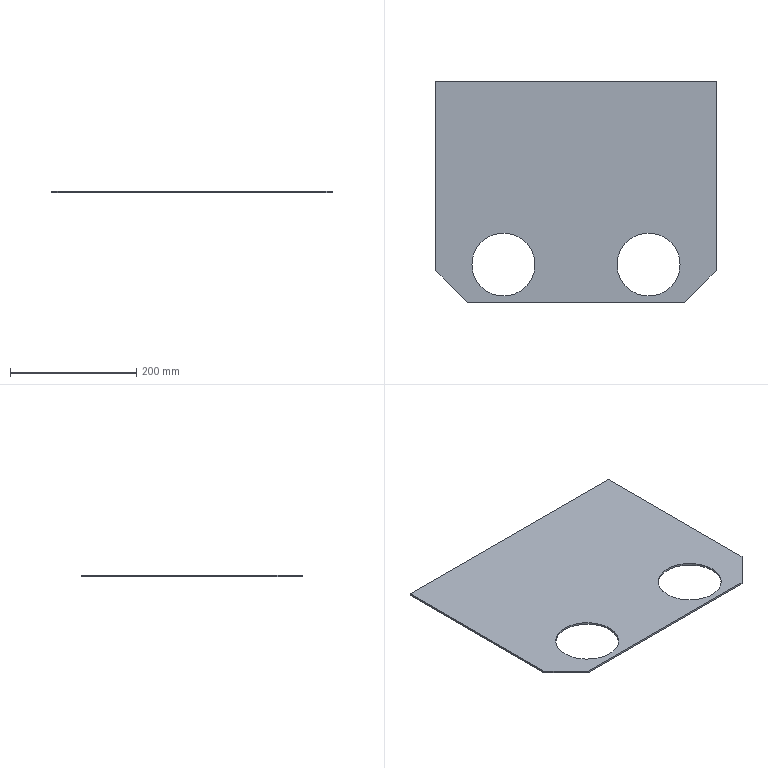Part | SolidWorks | features FlatPattern 1, SMBaseFlange 1, SheetMetal 1 | 1 solid | 12 faces | box 444 x 350 x 3 mm | volume 411576 mm3 | plane 8 | cylinder 4 | commonest cylinder face diameters 100 x4
STEP:
#1=CARTESIAN_POINT('',(65.,-115.,3.));
#2=VERTEX_POINT('',#1);
#3=CARTESIAN_POINT('',(165.,-115.,3.));
#4=VERTEX_POINT('',#3);
#5=CARTESIAN_POINT('',(115.,-115.,3.));
#6=DIRECTION('',(0.,0.,1.));
#7=DIRECTION('',(-1.,0.,0.));
#8=AXIS2_PLACEMENT_3D('',#5,#6,#7);
#9=CIRCLE('',#8,50.);
#10=EDGE_CURVE('',#2,#4,#9,.T.);
#11=ORIENTED_EDGE('',*,*,#10,.T.);
#12=CARTESIAN_POINT('',(165.,-115.,0.));
#13=VERTEX_POINT('',#12);
#14=CARTESIAN_POINT('',(165.,-115.,3.));
#15=DIRECTION('',(0.,0.,-1.));
#16=VECTOR('',#15,1000.);
#17=LINE('',#14,#16);
#18=EDGE_CURVE('',#4,#13,#17,.T.);
#19=ORIENTED_EDGE('',*,*,#18,.T.);
#20=CARTESIAN_POINT('',(65.,-115.,0.));
#21=VERTEX_POINT('',#20);
#22=CARTESIAN_POINT('',(115.,-115.,0.));
#23=DIRECTION('',(0.,0.,1.));
#24=DIRECTION('',(-1.,0.,0.));
#25=AXIS2_PLACEMENT_3D('',#22,#23,#24);
#26=CIRCLE('',#25,50.);
#27=EDGE_CURVE('',#21,#13,#26,.T.);
#28=ORIENTED_EDGE('',*,*,#27,.F.);
#29=CARTESIAN_POINT('',(65.,-115.,3.));
#30=DIRECTION('',(0.,0.,-1.));
#31=VECTOR('',#30,1000.);
#32=LINE('',#29,#31);
#33=EDGE_CURVE('',#2,#21,#32,.T.);
#34=ORIENTED_EDGE('',*,*,#33,.F.);
#35=EDGE_LOOP('',(#11,#19,#28,#34));
#36=FACE_OUTER_BOUND('',#35,.T.);
#37=CARTESIAN_POINT('',(115.,-115.,3.));
#38=DIRECTION('',(0.,0.,-1.));
#39=DIRECTION('',(-1.,0.,0.));
#40=AXIS2_PLACEMENT_3D('',#37,#38,#39);
#41=CYLINDRICAL_SURFACE('',#40,50.);
#42=ADVANCED_FACE('',(#36),#41,.F.);
#43=CARTESIAN_POINT('',(-165.,-115.,3.));
#44=VERTEX_POINT('',#43);
#45=CARTESIAN_POINT('',(-65.,-115.,3.));
#46=VERTEX_POINT('',#45);
#47=CARTESIAN_POINT('',(-115.,-115.,3.));
#48=DIRECTION('',(0.,0.,1.));
#49=DIRECTION('',(1.,0.,0.));
#50=AXIS2_PLACEMENT_3D('',#47,#48,#49);
#51=CIRCLE('',#50,50.);
#52=EDGE_CURVE('',#44,#46,#51,.T.);
#53=ORIENTED_EDGE('',*,*,#52,.T.);
#54=CARTESIAN_POINT('',(-65.,-115.,0.));
#55=VERTEX_POINT('',#54);
#56=CARTESIAN_POINT('',(-65.,-115.,3.));
#57=DIRECTION('',(0.,0.,-1.));
#58=VECTOR('',#57,1000.);
#59=LINE('',#56,#58);
#60=EDGE_CURVE('',#46,#55,#59,.T.);
#61=ORIENTED_EDGE('',*,*,#60,.T.);
#62=CARTESIAN_POINT('',(-165.,-115.,0.));
#63=VERTEX_POINT('',#62);
#64=CARTESIAN_POINT('',(-115.,-115.,0.));
#65=DIRECTION('',(0.,0.,1.));
#66=DIRECTION('',(1.,0.,0.));
#67=AXIS2_PLACEMENT_3D('',#64,#65,#66);
#68=CIRCLE('',#67,50.);
#69=EDGE_CURVE('',#63,#55,#68,.T.);
#70=ORIENTED_EDGE('',*,*,#69,.F.);
#71=CARTESIAN_POINT('',(-165.,-115.,3.));
#72=DIRECTION('',(0.,0.,-1.));
#73=VECTOR('',#72,1000.);
#74=LINE('',#71,#73);
#75=EDGE_CURVE('',#44,#63,#74,.T.);
#76=ORIENTED_EDGE('',*,*,#75,.F.);
#77=EDGE_LOOP('',(#53,#61,#70,#76));
#78=FACE_OUTER_BOUND('',#77,.T.);
#79=CARTESIAN_POINT('',(-115.,-115.,3.));
#80=DIRECTION('',(0.,0.,-1.));
#81=DIRECTION('',(-1.,0.,0.));
#82=AXIS2_PLACEMENT_3D('',#79,#80,#81);
#83=CYLINDRICAL_SURFACE('',#82,50.);
#84=ADVANCED_FACE('',(#78),#83,.F.);
#85=ORIENTED_EDGE('',*,*,#52,.F.);
#86=CARTESIAN_POINT('',(-115.,-115.,3.));
#87=DIRECTION('',(0.,0.,1.));
#88=DIRECTION('',(1.,0.,0.));
#89=AXIS2_PLACEMENT_3D('',#86,#87,#88);
#90=CIRCLE('',#89,50.);
#91=EDGE_CURVE('',#46,#44,#90,.T.);
#92=ORIENTED_EDGE('',*,*,#91,.F.);
#93=EDGE_LOOP('',(#85,#92));
#94=FACE_BOUND('',#93,.T.);
#95=CARTESIAN_POINT('',(-222.,175.,3.));
#96=VERTEX_POINT('',#95);
#97=CARTESIAN_POINT('',(-222.,-125.,3.));
#98=VERTEX_POINT('',#97);
#99=CARTESIAN_POINT('',(-222.,175.,3.));
#100=DIRECTION('',(0.,-1.,0.));
#101=VECTOR('',#100,1000.);
#102=LINE('',#99,#101);
#103=EDGE_CURVE('',#96,#98,#102,.T.);
#104=ORIENTED_EDGE('',*,*,#103,.T.);
#105=CARTESIAN_POINT('',(-172.,-175.,3.));
#106=VERTEX_POINT('',#105);
#107=CARTESIAN_POINT('',(-222.,-125.,3.));
#108=DIRECTION('',(0.7071,-0.7071,0.));
#109=VECTOR('',#108,1000.);
#110=LINE('',#107,#109);
#111=EDGE_CURVE('',#98,#106,#110,.T.);
#112=ORIENTED_EDGE('',*,*,#111,.T.);
#113=CARTESIAN_POINT('',(172.,-175.,3.));
#114=VERTEX_POINT('',#113);
#115=CARTESIAN_POINT('',(-172.,-175.,3.));
#116=DIRECTION('',(1.,0.,0.));
#117=VECTOR('',#116,1000.);
#118=LINE('',#115,#117);
#119=EDGE_CURVE('',#106,#114,#118,.T.);
#120=ORIENTED_EDGE('',*,*,#119,.T.);
#121=CARTESIAN_POINT('',(222.,-125.,3.));
#122=VERTEX_POINT('',#121);
#123=CARTESIAN_POINT('',(172.,-175.,3.));
#124=DIRECTION('',(0.7071,0.7071,0.));
#125=VECTOR('',#124,1000.);
#126=LINE('',#123,#125);
#127=EDGE_CURVE('',#114,#122,#126,.T.);
#128=ORIENTED_EDGE('',*,*,#127,.T.);
#129=CARTESIAN_POINT('',(222.,175.,3.));
#130=VERTEX_POINT('',#129);
#131=CARTESIAN_POINT('',(222.,175.,3.));
#132=DIRECTION('',(0.,1.,0.));
#133=VECTOR('',#132,1000.);
#134=LINE('',#131,#133);
#135=EDGE_CURVE('',#122,#130,#134,.T.);
#136=ORIENTED_EDGE('',*,*,#135,.T.);
#137=CARTESIAN_POINT('',(-222.,175.,3.));
#138=DIRECTION('',(-1.,0.,0.));
#139=VECTOR('',#138,1000.);
#140=LINE('',#137,#139);
#141=EDGE_CURVE('',#130,#96,#140,.T.);
#142=ORIENTED_EDGE('',*,*,#141,.T.);
#143=EDGE_LOOP('',(#104,#112,#120,#128,#136,#142));
#144=FACE_OUTER_BOUND('',#143,.T.);
#145=ORIENTED_EDGE('',*,*,#10,.F.);
#146=CARTESIAN_POINT('',(115.,-115.,3.));
#147=DIRECTION('',(0.,0.,1.));
#148=DIRECTION('',(-1.,0.,0.));
#149=AXIS2_PLACEMENT_3D('',#146,#147,#148);
#150=CIRCLE('',#149,50.);
#151=EDGE_CURVE('',#4,#2,#150,.T.);
#152=ORIENTED_EDGE('',*,*,#151,.F.);
#153=EDGE_LOOP('',(#145,#152));
#154=FACE_BOUND('',#153,.T.);
#155=CARTESIAN_POINT('',(0.,0.,3.));
#156=DIRECTION('',(0.,0.,1.));
#157=DIRECTION('',(1.,0.,0.));
#158=AXIS2_PLACEMENT_3D('',#155,#156,#157);
#159=PLANE('',#158);
#160=ADVANCED_FACE('',(#94,#144,#154),#159,.T.);
#161=CARTESIAN_POINT('',(-222.,175.,0.));
#162=VERTEX_POINT('',#161);
#163=CARTESIAN_POINT('',(-222.,-125.,0.));
#164=VERTEX_POINT('',#163);
#165=CARTESIAN_POINT('',(-222.,175.,0.));
#166=DIRECTION('',(0.,-1.,0.));
#167=VECTOR('',#166,1000.);
#168=LINE('',#165,#167);
#169=EDGE_CURVE('',#162,#164,#168,.T.);
#170=ORIENTED_EDGE('',*,*,#169,.F.);
#171=CARTESIAN_POINT('',(222.,175.,0.));
#172=VERTEX_POINT('',#171);
#173=CARTESIAN_POINT('',(-222.,175.,0.));
#174=DIRECTION('',(-1.,0.,0.));
#175=VECTOR('',#174,1000.);
#176=LINE('',#173,#175);
#177=EDGE_CURVE('',#172,#162,#176,.T.);
#178=ORIENTED_EDGE('',*,*,#177,.F.);
#179=CARTESIAN_POINT('',(222.,-125.,0.));
#180=VERTEX_POINT('',#179);
#181=CARTESIAN_POINT('',(222.,175.,0.));
#182=DIRECTION('',(0.,1.,0.));
#183=VECTOR('',#182,1000.);
#184=LINE('',#181,#183);
#185=EDGE_CURVE('',#180,#172,#184,.T.);
#186=ORIENTED_EDGE('',*,*,#185,.F.);
#187=CARTESIAN_POINT('',(172.,-175.,0.));
#188=VERTEX_POINT('',#187);
#189=CARTESIAN_POINT('',(172.,-175.,0.));
#190=DIRECTION('',(0.7071,0.7071,0.));
#191=VECTOR('',#190,1000.);
#192=LINE('',#189,#191);
#193=EDGE_CURVE('',#188,#180,#192,.T.);
#194=ORIENTED_EDGE('',*,*,#193,.F.);
#195=CARTESIAN_POINT('',(-172.,-175.,0.));
#196=VERTEX_POINT('',#195);
#197=CARTESIAN_POINT('',(-172.,-175.,0.));
#198=DIRECTION('',(1.,0.,0.));
#199=VECTOR('',#198,1000.);
#200=LINE('',#197,#199);
#201=EDGE_CURVE('',#196,#188,#200,.T.);
#202=ORIENTED_EDGE('',*,*,#201,.F.);
#203=CARTESIAN_POINT('',(-222.,-125.,0.));
#204=DIRECTION('',(0.7071,-0.7071,0.));
#205=VECTOR('',#204,1000.);
#206=LINE('',#203,#205);
#207=EDGE_CURVE('',#164,#196,#206,.T.);
#208=ORIENTED_EDGE('',*,*,#207,.F.);
#209=EDGE_LOOP('',(#170,#178,#186,#194,#202,#208));
#210=FACE_OUTER_BOUND('',#209,.T.);
#211=ORIENTED_EDGE('',*,*,#69,.T.);
#212=CARTESIAN_POINT('',(-115.,-115.,0.));
#213=DIRECTION('',(0.,0.,1.));
#214=DIRECTION('',(1.,0.,0.));
#215=AXIS2_PLACEMENT_3D('',#212,#213,#214);
#216=CIRCLE('',#215,50.);
#217=EDGE_CURVE('',#55,#63,#216,.T.);
#218=ORIENTED_EDGE('',*,*,#217,.T.);
#219=EDGE_LOOP('',(#211,#218));
#220=FACE_BOUND('',#219,.T.);
#221=ORIENTED_EDGE('',*,*,#27,.T.);
#222=CARTESIAN_POINT('',(115.,-115.,0.));
#223=DIRECTION('',(0.,0.,1.));
#224=DIRECTION('',(-1.,0.,0.));
#225=AXIS2_PLACEMENT_3D('',#222,#223,#224);
#226=CIRCLE('',#225,50.);
#227=EDGE_CURVE('',#13,#21,#226,.T.);
#228=ORIENTED_EDGE('',*,*,#227,.T.);
#229=EDGE_LOOP('',(#221,#228));
#230=FACE_BOUND('',#229,.T.);
#231=CARTESIAN_POINT('',(0.,0.,0.));
#232=DIRECTION('',(0.,0.,1.));
#233=DIRECTION('',(1.,0.,0.));
#234=AXIS2_PLACEMENT_3D('',#231,#232,#233);
#235=PLANE('',#234);
#236=ADVANCED_FACE('',(#210,#220,#230),#235,.F.);
#237=ORIENTED_EDGE('',*,*,#169,.T.);
#238=CARTESIAN_POINT('',(-222.,-125.,3.));
#239=DIRECTION('',(0.,0.,-1.));
#240=VECTOR('',#239,1000.);
#241=LINE('',#238,#240);
#242=EDGE_CURVE('',#98,#164,#241,.T.);
#243=ORIENTED_EDGE('',*,*,#242,.F.);
#244=ORIENTED_EDGE('',*,*,#103,.F.);
#245=CARTESIAN_POINT('',(-222.,175.,3.));
#246=DIRECTION('',(0.,0.,-1.));
#247=VECTOR('',#246,1000.);
#248=LINE('',#245,#247);
#249=EDGE_CURVE('',#96,#162,#248,.T.);
#250=ORIENTED_EDGE('',*,*,#249,.T.);
#251=EDGE_LOOP('',(#237,#243,#244,#250));
#252=FACE_OUTER_BOUND('',#251,.T.);
#253=CARTESIAN_POINT('',(-222.,175.,3.));
#254=DIRECTION('',(1.,0.,0.));
#255=DIRECTION('',(0.,1.,0.));
#256=AXIS2_PLACEMENT_3D('',#253,#254,#255);
#257=PLANE('',#256);
#258=ADVANCED_FACE('',(#252),#257,.F.);
#259=ORIENTED_EDGE('',*,*,#207,.T.);
#260=CARTESIAN_POINT('',(-172.,-175.,3.));
#261=DIRECTION('',(0.,0.,-1.));
#262=VECTOR('',#261,1000.);
#263=LINE('',#260,#262);
#264=EDGE_CURVE('',#106,#196,#263,.T.);
#265=ORIENTED_EDGE('',*,*,#264,.F.);
#266=ORIENTED_EDGE('',*,*,#111,.F.);
#267=ORIENTED_EDGE('',*,*,#242,.T.);
#268=EDGE_LOOP('',(#259,#265,#266,#267));
#269=FACE_OUTER_BOUND('',#268,.T.);
#270=CARTESIAN_POINT('',(-222.,-125.,3.));
#271=DIRECTION('',(0.7071,0.7071,0.));
#272=DIRECTION('',(-0.7071,0.7071,0.));
#273=AXIS2_PLACEMENT_3D('',#270,#271,#272);
#274=PLANE('',#273);
#275=ADVANCED_FACE('',(#269),#274,.F.);
#276=ORIENTED_EDGE('',*,*,#201,.T.);
#277=CARTESIAN_POINT('',(172.,-175.,3.));
#278=DIRECTION('',(0.,0.,-1.));
#279=VECTOR('',#278,1000.);
#280=LINE('',#277,#279);
#281=EDGE_CURVE('',#114,#188,#280,.T.);
#282=ORIENTED_EDGE('',*,*,#281,.F.);
#283=ORIENTED_EDGE('',*,*,#119,.F.);
#284=ORIENTED_EDGE('',*,*,#264,.T.);
#285=EDGE_LOOP('',(#276,#282,#283,#284));
#286=FACE_OUTER_BOUND('',#285,.T.);
#287=CARTESIAN_POINT('',(-172.,-175.,3.));
#288=DIRECTION('',(0.,1.,0.));
#289=DIRECTION('',(0.,0.,1.));
#290=AXIS2_PLACEMENT_3D('',#287,#288,#289);
#291=PLANE('',#290);
#292=ADVANCED_FACE('',(#286),#291,.F.);
#293=ORIENTED_EDGE('',*,*,#193,.T.);
#294=CARTESIAN_POINT('',(222.,-125.,3.));
#295=DIRECTION('',(0.,0.,-1.));
#296=VECTOR('',#295,1000.);
#297=LINE('',#294,#296);
#298=EDGE_CURVE('',#122,#180,#297,.T.);
#299=ORIENTED_EDGE('',*,*,#298,.F.);
#300=ORIENTED_EDGE('',*,*,#127,.F.);
#301=ORIENTED_EDGE('',*,*,#281,.T.);
#302=EDGE_LOOP('',(#293,#299,#300,#301));
#303=FACE_OUTER_BOUND('',#302,.T.);
#304=CARTESIAN_POINT('',(172.,-175.,3.));
#305=DIRECTION('',(-0.7071,0.7071,0.));
#306=DIRECTION('',(-0.7071,-0.7071,0.));
#307=AXIS2_PLACEMENT_3D('',#304,#305,#306);
#308=PLANE('',#307);
#309=ADVANCED_FACE('',(#303),#308,.F.);
#310=ORIENTED_EDGE('',*,*,#185,.T.);
#311=CARTESIAN_POINT('',(222.,175.,3.));
#312=DIRECTION('',(0.,0.,-1.));
#313=VECTOR('',#312,1000.);
#314=LINE('',#311,#313);
#315=EDGE_CURVE('',#130,#172,#314,.T.);
#316=ORIENTED_EDGE('',*,*,#315,.F.);
#317=ORIENTED_EDGE('',*,*,#135,.F.);
#318=ORIENTED_EDGE('',*,*,#298,.T.);
#319=EDGE_LOOP('',(#310,#316,#317,#318));
#320=FACE_OUTER_BOUND('',#319,.T.);
#321=CARTESIAN_POINT('',(222.,175.,3.));
#322=DIRECTION('',(-1.,0.,0.));
#323=DIRECTION('',(0.,-1.,0.));
#324=AXIS2_PLACEMENT_3D('',#321,#322,#323);
#325=PLANE('',#324);
#326=ADVANCED_FACE('',(#320),#325,.F.);
#327=ORIENTED_EDGE('',*,*,#177,.T.);
#328=ORIENTED_EDGE('',*,*,#249,.F.);
#329=ORIENTED_EDGE('',*,*,#141,.F.);
#330=ORIENTED_EDGE('',*,*,#315,.T.);
#331=EDGE_LOOP('',(#327,#328,#329,#330));
#332=FACE_OUTER_BOUND('',#331,.T.);
#333=CARTESIAN_POINT('',(-222.,175.,3.));
#334=DIRECTION('',(0.,-1.,0.));
#335=DIRECTION('',(0.,0.,-1.));
#336=AXIS2_PLACEMENT_3D('',#333,#334,#335);
#337=PLANE('',#336);
#338=ADVANCED_FACE('',(#332),#337,.F.);
#339=ORIENTED_EDGE('',*,*,#60,.F.);
#340=ORIENTED_EDGE('',*,*,#91,.T.);
#341=ORIENTED_EDGE('',*,*,#75,.T.);
#342=ORIENTED_EDGE('',*,*,#217,.F.);
#343=EDGE_LOOP('',(#339,#340,#341,#342));
#344=FACE_OUTER_BOUND('',#343,.T.);
#345=CARTESIAN_POINT('',(-115.,-115.,3.));
#346=DIRECTION('',(0.,0.,-1.));
#347=DIRECTION('',(-1.,0.,0.));
#348=AXIS2_PLACEMENT_3D('',#345,#346,#347);
#349=CYLINDRICAL_SURFACE('',#348,50.);
#350=ADVANCED_FACE('',(#344),#349,.F.);
#351=ORIENTED_EDGE('',*,*,#18,.F.);
#352=ORIENTED_EDGE('',*,*,#151,.T.);
#353=ORIENTED_EDGE('',*,*,#33,.T.);
#354=ORIENTED_EDGE('',*,*,#227,.F.);
#355=EDGE_LOOP('',(#351,#352,#353,#354));
#356=FACE_OUTER_BOUND('',#355,.T.);
#357=CARTESIAN_POINT('',(115.,-115.,3.));
#358=DIRECTION('',(0.,0.,-1.));
#359=DIRECTION('',(-1.,0.,0.));
#360=AXIS2_PLACEMENT_3D('',#357,#358,#359);
#361=CYLINDRICAL_SURFACE('',#360,50.);
#362=ADVANCED_FACE('',(#356),#361,.F.);
#363=CLOSED_SHELL('',(#42,#84,#160,#236,#258,#275,#292,#309,#326,#338,#350,#362));
#364=MANIFOLD_SOLID_BREP('',#363);
#365=CARTESIAN_POINT('',(0.,0.,0.));
#366=DIRECTION('',(0.,0.,1.));
#367=DIRECTION('',(1.,0.,0.));
#368=AXIS2_PLACEMENT_3D('',#365,#366,#367);
#369=(LENGTH_UNIT()NAMED_UNIT(*)SI_UNIT(.MILLI.,.METRE.));
#370=UNCERTAINTY_MEASURE_WITH_UNIT(LENGTH_MEASURE(0.00001),#369,'','');
#371=(NAMED_UNIT(*)PLANE_ANGLE_UNIT()SI_UNIT($,.RADIAN.));
#372=(NAMED_UNIT(*)SI_UNIT($,.STERADIAN.)SOLID_ANGLE_UNIT());
#373=(GEOMETRIC_REPRESENTATION_CONTEXT(3)GLOBAL_UNCERTAINTY_ASSIGNED_CONTEXT((#370))GLOBAL_UNIT_ASSIGNED_CONTEXT((#369,#371,#372))REPRESENTATION_CONTEXT('',''));
#374=ADVANCED_BREP_SHAPE_REPRESENTATION('',(#364,#368),#373);